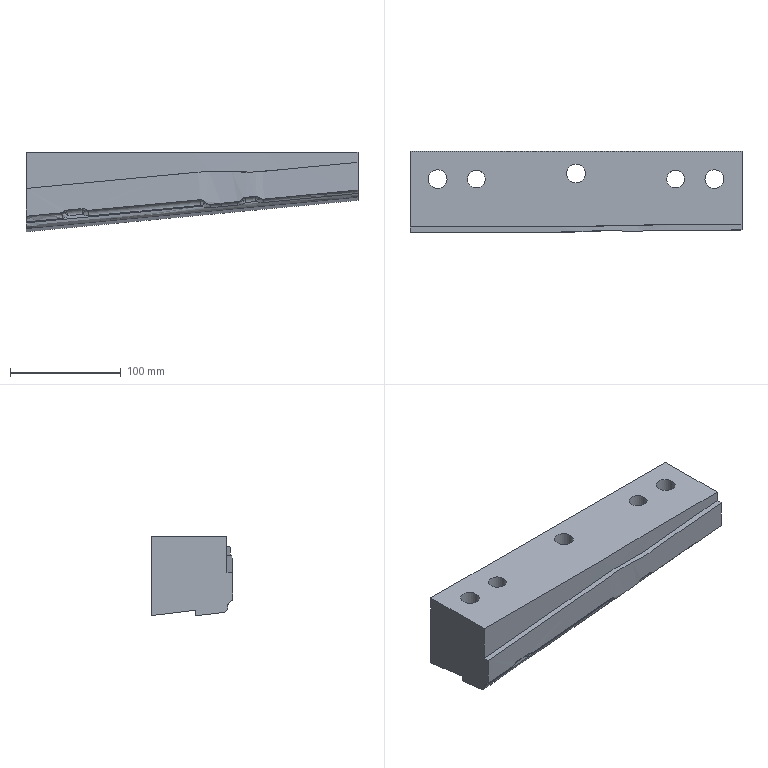Part | NX | features solid 2 | 1 solid | 43 faces | box 300 x 73.219 x 71.99 mm | volume 1084451 mm3 | spline 28 | cylinder 8 | plane 7 | commonest cylinder face diameters 17 x3 25 x3 16 x2